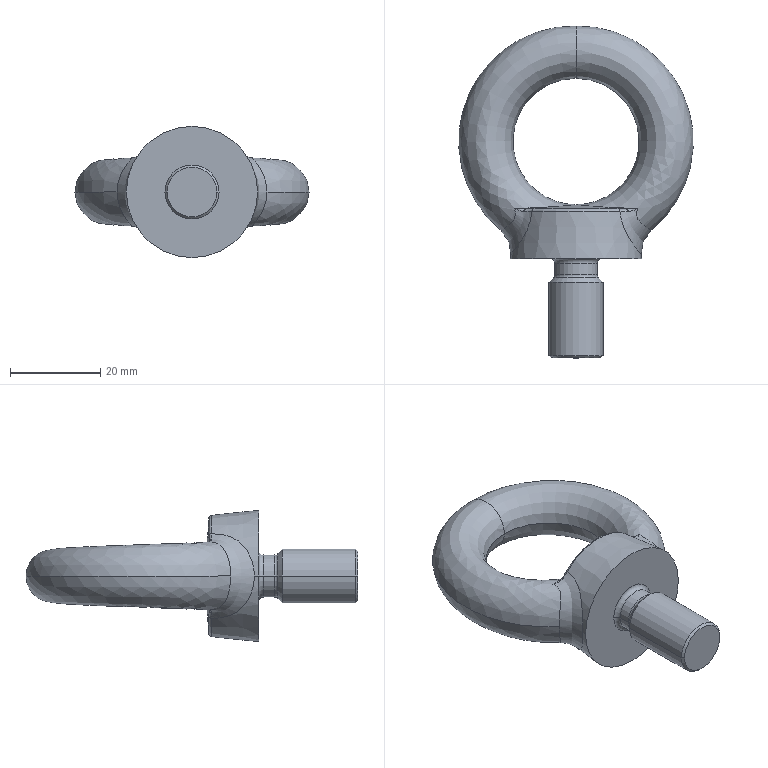Part | SolidWorks | features Fillet 5, Revolution 3, Chamfer 2, Blend 1, MirrorPattern 1 | 1 solid | 38 faces | box 52.011 x 73.603 x 29.1 mm | volume 21726 mm3 | spline 18 | cone 8 | torus 6 | cylinder 4 | plane 2 | commonest cylinder face diameters 9.4 x2 12 x2